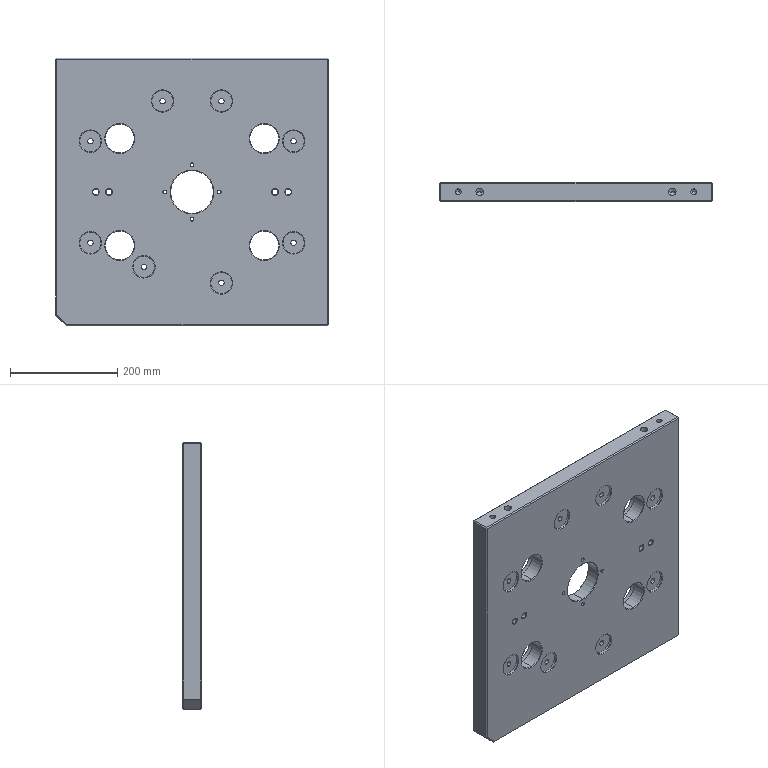Part | STEP file | PBS - 1 cav | 1 solid | 221 faces | box 510 x 36 x 500 mm | volume 8424078 mm3 | cylinder 92 | cone 86 | plane 43 | commonest cylinder face diameters 10.2 x16 40 x16 6.8 x8 10.5 x8 11 x8 14 x8